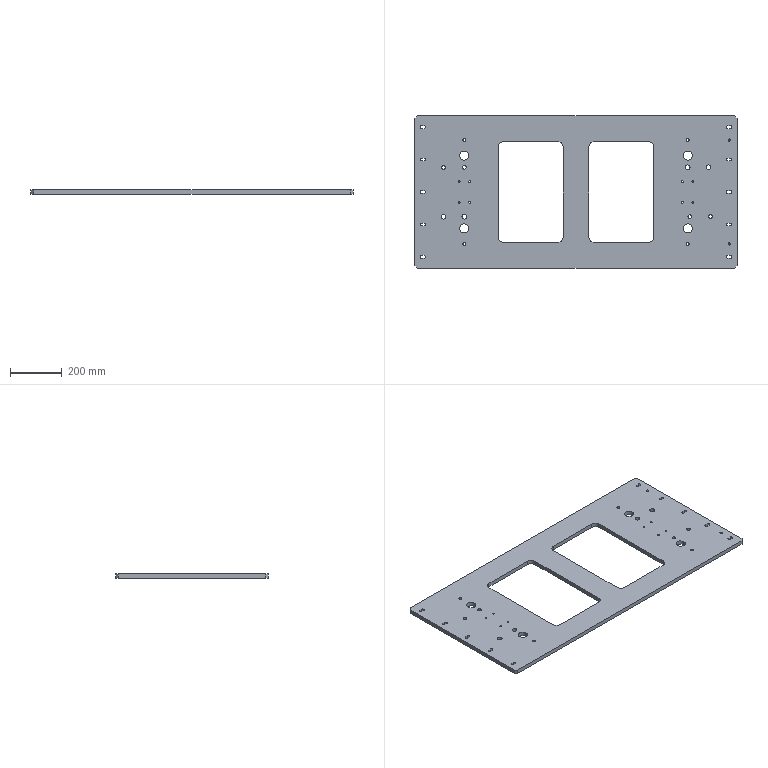Part | SolidWorks | features BaseBody 1 | 1 solid | 128 faces | box 1240 x 588 x 16 mm | volume 8435725 mm3 | cylinder 90 | plane 38 | commonest cylinder face diameters 11 x38 6.8 x16 14 x8 18.5 x8 35 x8 40 x8